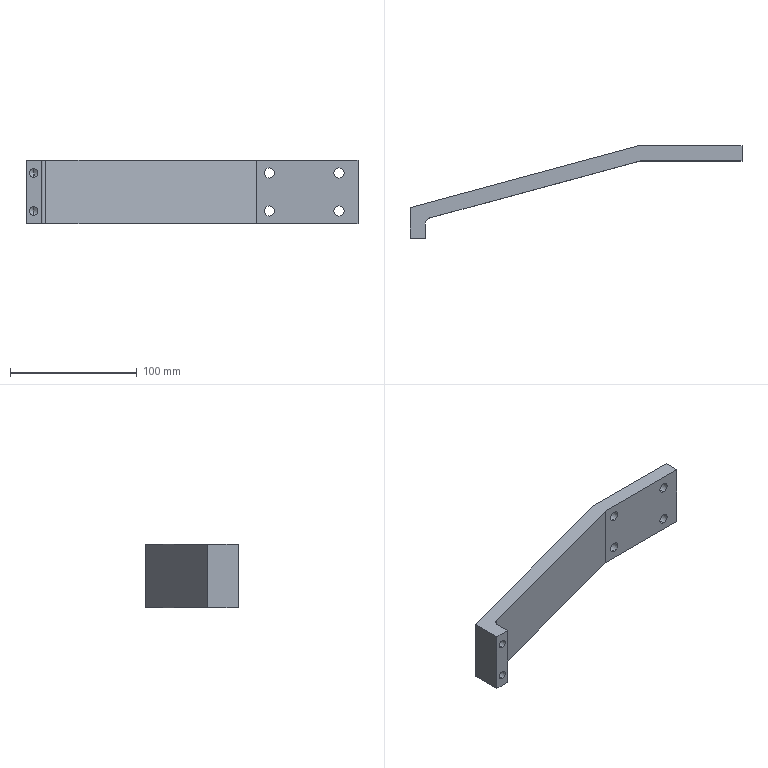Part | SolidWorks | features BaseBody 1 | 1 solid | 27 faces | box 262 x 73 x 50 mm | volume 165869 mm3 | cylinder 13 | plane 10 | cone 4 | commonest cylinder face diameters 8 x8 6.8 x4 10 x1
STEP:
#1=CARTESIAN_POINT('',(260.,-92.,221.121));
#2=VERTEX_POINT('',#1);
#3=CARTESIAN_POINT('',(260.,-92.,213.121));
#4=VERTEX_POINT('',#3);
#5=CARTESIAN_POINT('',(260.,-92.,217.121));
#6=DIRECTION('',(0.,-1.,0.));
#7=DIRECTION('',(0.,0.,1.));
#8=AXIS2_PLACEMENT_3D('',#5,#6,#7);
#9=CIRCLE('',#8,4.);
#10=EDGE_CURVE('',#2,#4,#9,.T.);
#11=ORIENTED_EDGE('',*,*,#10,.T.);
#12=CARTESIAN_POINT('',(260.,-80.,213.121));
#13=VERTEX_POINT('',#12);
#14=CARTESIAN_POINT('',(260.,-153.,213.121));
#15=DIRECTION('',(0.,1.,0.));
#16=VECTOR('',#15,1000.);
#17=LINE('',#14,#16);
#18=EDGE_CURVE('',#4,#13,#17,.T.);
#19=ORIENTED_EDGE('',*,*,#18,.T.);
#20=CARTESIAN_POINT('',(260.,-80.,221.121));
#21=VERTEX_POINT('',#20);
#22=CARTESIAN_POINT('',(260.,-80.,217.121));
#23=DIRECTION('',(0.,1.,0.));
#24=DIRECTION('',(0.,0.,1.));
#25=AXIS2_PLACEMENT_3D('',#22,#23,#24);
#26=CIRCLE('',#25,4.);
#27=EDGE_CURVE('',#13,#21,#26,.T.);
#28=ORIENTED_EDGE('',*,*,#27,.T.);
#29=CARTESIAN_POINT('',(260.,-153.,221.121));
#30=DIRECTION('',(0.,1.,0.));
#31=VECTOR('',#30,1000.);
#32=LINE('',#29,#31);
#33=EDGE_CURVE('',#2,#21,#32,.T.);
#34=ORIENTED_EDGE('',*,*,#33,.F.);
#35=EDGE_LOOP('',(#11,#19,#28,#34));
#36=FACE_OUTER_BOUND('',#35,.T.);
#37=CARTESIAN_POINT('',(260.,-153.,217.121));
#38=DIRECTION('',(0.,1.,0.));
#39=DIRECTION('',(0.,0.,1.));
#40=AXIS2_PLACEMENT_3D('',#37,#38,#39);
#41=CYLINDRICAL_SURFACE('',#40,4.);
#42=ADVANCED_FACE('',(#36),#41,.F.);
#43=CARTESIAN_POINT('',(260.,-92.,251.121));
#44=VERTEX_POINT('',#43);
#45=CARTESIAN_POINT('',(260.,-92.,243.121));
#46=VERTEX_POINT('',#45);
#47=CARTESIAN_POINT('',(260.,-92.,247.121));
#48=DIRECTION('',(0.,-1.,0.));
#49=DIRECTION('',(0.,0.,1.));
#50=AXIS2_PLACEMENT_3D('',#47,#48,#49);
#51=CIRCLE('',#50,4.);
#52=EDGE_CURVE('',#44,#46,#51,.T.);
#53=ORIENTED_EDGE('',*,*,#52,.T.);
#54=CARTESIAN_POINT('',(260.,-80.,243.121));
#55=VERTEX_POINT('',#54);
#56=CARTESIAN_POINT('',(260.,-153.,243.121));
#57=DIRECTION('',(0.,1.,0.));
#58=VECTOR('',#57,1000.);
#59=LINE('',#56,#58);
#60=EDGE_CURVE('',#46,#55,#59,.T.);
#61=ORIENTED_EDGE('',*,*,#60,.T.);
#62=CARTESIAN_POINT('',(260.,-80.,251.121));
#63=VERTEX_POINT('',#62);
#64=CARTESIAN_POINT('',(260.,-80.,247.121));
#65=DIRECTION('',(0.,1.,0.));
#66=DIRECTION('',(0.,0.,1.));
#67=AXIS2_PLACEMENT_3D('',#64,#65,#66);
#68=CIRCLE('',#67,4.);
#69=EDGE_CURVE('',#55,#63,#68,.T.);
#70=ORIENTED_EDGE('',*,*,#69,.T.);
#71=CARTESIAN_POINT('',(260.,-153.,251.121));
#72=DIRECTION('',(0.,1.,0.));
#73=VECTOR('',#72,1000.);
#74=LINE('',#71,#73);
#75=EDGE_CURVE('',#44,#63,#74,.T.);
#76=ORIENTED_EDGE('',*,*,#75,.F.);
#77=EDGE_LOOP('',(#53,#61,#70,#76));
#78=FACE_OUTER_BOUND('',#77,.T.);
#79=CARTESIAN_POINT('',(260.,-153.,247.121));
#80=DIRECTION('',(0.,1.,0.));
#81=DIRECTION('',(0.,0.,1.));
#82=AXIS2_PLACEMENT_3D('',#79,#80,#81);
#83=CYLINDRICAL_SURFACE('',#82,4.);
#84=ADVANCED_FACE('',(#78),#83,.F.);
#85=CARTESIAN_POINT('',(315.,-92.,251.121));
#86=VERTEX_POINT('',#85);
#87=CARTESIAN_POINT('',(315.,-92.,243.121));
#88=VERTEX_POINT('',#87);
#89=CARTESIAN_POINT('',(315.,-92.,247.121));
#90=DIRECTION('',(0.,-1.,0.));
#91=DIRECTION('',(0.,0.,1.));
#92=AXIS2_PLACEMENT_3D('',#89,#90,#91);
#93=CIRCLE('',#92,4.);
#94=EDGE_CURVE('',#86,#88,#93,.T.);
#95=ORIENTED_EDGE('',*,*,#94,.T.);
#96=CARTESIAN_POINT('',(315.,-80.,243.121));
#97=VERTEX_POINT('',#96);
#98=CARTESIAN_POINT('',(315.,-153.,243.121));
#99=DIRECTION('',(0.,1.,0.));
#100=VECTOR('',#99,1000.);
#101=LINE('',#98,#100);
#102=EDGE_CURVE('',#88,#97,#101,.T.);
#103=ORIENTED_EDGE('',*,*,#102,.T.);
#104=CARTESIAN_POINT('',(315.,-80.,251.121));
#105=VERTEX_POINT('',#104);
#106=CARTESIAN_POINT('',(315.,-80.,247.121));
#107=DIRECTION('',(0.,1.,0.));
#108=DIRECTION('',(0.,0.,1.));
#109=AXIS2_PLACEMENT_3D('',#106,#107,#108);
#110=CIRCLE('',#109,4.);
#111=EDGE_CURVE('',#97,#105,#110,.T.);
#112=ORIENTED_EDGE('',*,*,#111,.T.);
#113=CARTESIAN_POINT('',(315.,-153.,251.121));
#114=DIRECTION('',(0.,1.,0.));
#115=VECTOR('',#114,1000.);
#116=LINE('',#113,#115);
#117=EDGE_CURVE('',#86,#105,#116,.T.);
#118=ORIENTED_EDGE('',*,*,#117,.F.);
#119=EDGE_LOOP('',(#95,#103,#112,#118));
#120=FACE_OUTER_BOUND('',#119,.T.);
#121=CARTESIAN_POINT('',(315.,-153.,247.121));
#122=DIRECTION('',(0.,1.,0.));
#123=DIRECTION('',(0.,0.,1.));
#124=AXIS2_PLACEMENT_3D('',#121,#122,#123);
#125=CYLINDRICAL_SURFACE('',#124,4.);
#126=ADVANCED_FACE('',(#120),#125,.F.);
#127=CARTESIAN_POINT('',(315.,-92.,221.121));
#128=VERTEX_POINT('',#127);
#129=CARTESIAN_POINT('',(315.,-92.,213.121));
#130=VERTEX_POINT('',#129);
#131=CARTESIAN_POINT('',(315.,-92.,217.121));
#132=DIRECTION('',(0.,-1.,0.));
#133=DIRECTION('',(0.,0.,1.));
#134=AXIS2_PLACEMENT_3D('',#131,#132,#133);
#135=CIRCLE('',#134,4.);
#136=EDGE_CURVE('',#128,#130,#135,.T.);
#137=ORIENTED_EDGE('',*,*,#136,.T.);
#138=CARTESIAN_POINT('',(315.,-80.,213.121));
#139=VERTEX_POINT('',#138);
#140=CARTESIAN_POINT('',(315.,-153.,213.121));
#141=DIRECTION('',(0.,1.,0.));
#142=VECTOR('',#141,1000.);
#143=LINE('',#140,#142);
#144=EDGE_CURVE('',#130,#139,#143,.T.);
#145=ORIENTED_EDGE('',*,*,#144,.T.);
#146=CARTESIAN_POINT('',(315.,-80.,221.121));
#147=VERTEX_POINT('',#146);
#148=CARTESIAN_POINT('',(315.,-80.,217.121));
#149=DIRECTION('',(0.,1.,0.));
#150=DIRECTION('',(0.,0.,1.));
#151=AXIS2_PLACEMENT_3D('',#148,#149,#150);
#152=CIRCLE('',#151,4.);
#153=EDGE_CURVE('',#139,#147,#152,.T.);
#154=ORIENTED_EDGE('',*,*,#153,.T.);
#155=CARTESIAN_POINT('',(315.,-153.,221.121));
#156=DIRECTION('',(0.,1.,0.));
#157=VECTOR('',#156,1000.);
#158=LINE('',#155,#157);
#159=EDGE_CURVE('',#128,#147,#158,.T.);
#160=ORIENTED_EDGE('',*,*,#159,.F.);
#161=EDGE_LOOP('',(#137,#145,#154,#160));
#162=FACE_OUTER_BOUND('',#161,.T.);
#163=CARTESIAN_POINT('',(315.,-153.,217.121));
#164=DIRECTION('',(0.,1.,0.));
#165=DIRECTION('',(0.,0.,1.));
#166=AXIS2_PLACEMENT_3D('',#163,#164,#165);
#167=CYLINDRICAL_SURFACE('',#166,4.);
#168=ADVANCED_FACE('',(#162),#167,.F.);
#169=CARTESIAN_POINT('',(74.,-140.,250.521));
#170=VERTEX_POINT('',#169);
#171=CARTESIAN_POINT('',(74.,-140.,243.721));
#172=VERTEX_POINT('',#171);
#173=CARTESIAN_POINT('',(74.,-140.,247.121));
#174=DIRECTION('',(0.,-1.,0.));
#175=DIRECTION('',(0.,0.,-1.));
#176=AXIS2_PLACEMENT_3D('',#173,#174,#175);
#177=CIRCLE('',#176,3.4);
#178=EDGE_CURVE('',#170,#172,#177,.T.);
#179=ORIENTED_EDGE('',*,*,#178,.F.);
#180=CARTESIAN_POINT('',(74.,-153.,250.521));
#181=VERTEX_POINT('',#180);
#182=CARTESIAN_POINT('',(74.,-153.,250.521));
#183=DIRECTION('',(0.,-1.,0.));
#184=VECTOR('',#183,1000.);
#185=LINE('',#182,#184);
#186=EDGE_CURVE('',#170,#181,#185,.T.);
#187=ORIENTED_EDGE('',*,*,#186,.T.);
#188=CARTESIAN_POINT('',(74.,-153.,243.721));
#189=VERTEX_POINT('',#188);
#190=CARTESIAN_POINT('',(74.,-153.,247.121));
#191=DIRECTION('',(0.,-1.,0.));
#192=DIRECTION('',(0.,0.,-1.));
#193=AXIS2_PLACEMENT_3D('',#190,#191,#192);
#194=CIRCLE('',#193,3.4);
#195=EDGE_CURVE('',#181,#189,#194,.T.);
#196=ORIENTED_EDGE('',*,*,#195,.T.);
#197=CARTESIAN_POINT('',(74.,-153.,243.721));
#198=DIRECTION('',(0.,-1.,0.));
#199=VECTOR('',#198,1000.);
#200=LINE('',#197,#199);
#201=EDGE_CURVE('',#172,#189,#200,.T.);
#202=ORIENTED_EDGE('',*,*,#201,.F.);
#203=EDGE_LOOP('',(#179,#187,#196,#202));
#204=FACE_OUTER_BOUND('',#203,.T.);
#205=CARTESIAN_POINT('',(74.,-153.,247.121));
#206=DIRECTION('',(0.,-1.,0.));
#207=DIRECTION('',(0.,0.,-1.));
#208=AXIS2_PLACEMENT_3D('',#205,#206,#207);
#209=CYLINDRICAL_SURFACE('',#208,3.4);
#210=ADVANCED_FACE('',(#204),#209,.F.);
#211=CARTESIAN_POINT('',(74.,-140.,220.521));
#212=VERTEX_POINT('',#211);
#213=CARTESIAN_POINT('',(74.,-140.,213.721));
#214=VERTEX_POINT('',#213);
#215=CARTESIAN_POINT('',(74.,-140.,217.121));
#216=DIRECTION('',(0.,-1.,0.));
#217=DIRECTION('',(0.,0.,-1.));
#218=AXIS2_PLACEMENT_3D('',#215,#216,#217);
#219=CIRCLE('',#218,3.4);
#220=EDGE_CURVE('',#212,#214,#219,.T.);
#221=ORIENTED_EDGE('',*,*,#220,.F.);
#222=CARTESIAN_POINT('',(74.,-153.,220.521));
#223=VERTEX_POINT('',#222);
#224=CARTESIAN_POINT('',(74.,-153.,220.521));
#225=DIRECTION('',(0.,-1.,0.));
#226=VECTOR('',#225,1000.);
#227=LINE('',#224,#226);
#228=EDGE_CURVE('',#212,#223,#227,.T.);
#229=ORIENTED_EDGE('',*,*,#228,.T.);
#230=CARTESIAN_POINT('',(74.,-153.,213.721));
#231=VERTEX_POINT('',#230);
#232=CARTESIAN_POINT('',(74.,-153.,217.121));
#233=DIRECTION('',(0.,-1.,0.));
#234=DIRECTION('',(0.,0.,-1.));
#235=AXIS2_PLACEMENT_3D('',#232,#233,#234);
#236=CIRCLE('',#235,3.4);
#237=EDGE_CURVE('',#223,#231,#236,.T.);
#238=ORIENTED_EDGE('',*,*,#237,.T.);
#239=CARTESIAN_POINT('',(74.,-153.,213.721));
#240=DIRECTION('',(0.,-1.,0.));
#241=VECTOR('',#240,1000.);
#242=LINE('',#239,#241);
#243=EDGE_CURVE('',#214,#231,#242,.T.);
#244=ORIENTED_EDGE('',*,*,#243,.F.);
#245=EDGE_LOOP('',(#221,#229,#238,#244));
#246=FACE_OUTER_BOUND('',#245,.T.);
#247=CARTESIAN_POINT('',(74.,-153.,217.121));
#248=DIRECTION('',(0.,-1.,0.));
#249=DIRECTION('',(0.,0.,-1.));
#250=AXIS2_PLACEMENT_3D('',#247,#248,#249);
#251=CYLINDRICAL_SURFACE('',#250,3.4);
#252=ADVANCED_FACE('',(#246),#251,.F.);
#253=CARTESIAN_POINT('',(74.,-137.957,247.121));
#254=VERTEX_POINT('',#253);
#255=CARTESIAN_POINT('',(74.,-140.,243.721));
#256=DIRECTION('',(0.,-0.515,-0.8572));
#257=VECTOR('',#256,1000.);
#258=LINE('',#255,#257);
#259=EDGE_CURVE('',#254,#172,#258,.T.);
#260=ORIENTED_EDGE('',*,*,#259,.F.);
#261=CARTESIAN_POINT('',(74.,-140.,250.521));
#262=DIRECTION('',(0.,-0.515,0.8572));
#263=VECTOR('',#262,1000.);
#264=LINE('',#261,#263);
#265=EDGE_CURVE('',#254,#170,#264,.T.);
#266=ORIENTED_EDGE('',*,*,#265,.T.);
#267=ORIENTED_EDGE('',*,*,#178,.T.);
#268=EDGE_LOOP('',(#260,#266,#267));
#269=FACE_OUTER_BOUND('',#268,.T.);
#270=CARTESIAN_POINT('',(74.,-140.,247.121));
#271=DIRECTION('',(0.,-1.,0.));
#272=DIRECTION('',(0.,0.,-1.));
#273=AXIS2_PLACEMENT_3D('',#270,#271,#272);
#274=CONICAL_SURFACE('',#273,3.4,1.03);
#275=ADVANCED_FACE('',(#269),#274,.F.);
#276=CARTESIAN_POINT('',(74.,-137.957,217.121));
#277=VERTEX_POINT('',#276);
#278=CARTESIAN_POINT('',(74.,-140.,213.721));
#279=DIRECTION('',(0.,-0.515,-0.8572));
#280=VECTOR('',#279,1000.);
#281=LINE('',#278,#280);
#282=EDGE_CURVE('',#277,#214,#281,.T.);
#283=ORIENTED_EDGE('',*,*,#282,.F.);
#284=CARTESIAN_POINT('',(74.,-140.,220.521));
#285=DIRECTION('',(0.,-0.515,0.8572));
#286=VECTOR('',#285,1000.);
#287=LINE('',#284,#286);
#288=EDGE_CURVE('',#277,#212,#287,.T.);
#289=ORIENTED_EDGE('',*,*,#288,.T.);
#290=ORIENTED_EDGE('',*,*,#220,.T.);
#291=EDGE_LOOP('',(#283,#289,#290));
#292=FACE_OUTER_BOUND('',#291,.T.);
#293=CARTESIAN_POINT('',(74.,-140.,217.121));
#294=DIRECTION('',(0.,-1.,0.));
#295=DIRECTION('',(0.,0.,-1.));
#296=AXIS2_PLACEMENT_3D('',#293,#294,#295);
#297=CONICAL_SURFACE('',#296,3.4,1.03);
#298=ADVANCED_FACE('',(#292),#297,.F.);
#299=CARTESIAN_POINT('',(248.405,-80.,207.121));
#300=VERTEX_POINT('',#299);
#301=CARTESIAN_POINT('',(248.405,-80.,257.121));
#302=VERTEX_POINT('',#301);
#303=CARTESIAN_POINT('',(248.405,-80.,207.121));
#304=DIRECTION('',(0.,0.,1.));
#305=VECTOR('',#304,1000.);
#306=LINE('',#303,#305);
#307=EDGE_CURVE('',#300,#302,#306,.T.);
#308=ORIENTED_EDGE('',*,*,#307,.F.);
#309=CARTESIAN_POINT('',(68.,-128.816,207.121));
#310=VERTEX_POINT('',#309);
#311=CARTESIAN_POINT('',(68.,-128.816,207.121));
#312=DIRECTION('',(0.9653,0.2612,0.));
#313=VECTOR('',#312,1000.);
#314=LINE('',#311,#313);
#315=EDGE_CURVE('',#310,#300,#314,.T.);
#316=ORIENTED_EDGE('',*,*,#315,.F.);
#317=CARTESIAN_POINT('',(68.,-128.816,257.121));
#318=VERTEX_POINT('',#317);
#319=CARTESIAN_POINT('',(68.,-128.816,207.121));
#320=DIRECTION('',(0.,0.,-1.));
#321=VECTOR('',#320,1000.);
#322=LINE('',#319,#321);
#323=EDGE_CURVE('',#318,#310,#322,.T.);
#324=ORIENTED_EDGE('',*,*,#323,.F.);
#325=CARTESIAN_POINT('',(68.,-128.816,257.121));
#326=DIRECTION('',(-0.9653,-0.2612,0.));
#327=VECTOR('',#326,1000.);
#328=LINE('',#325,#327);
#329=EDGE_CURVE('',#302,#318,#328,.T.);
#330=ORIENTED_EDGE('',*,*,#329,.F.);
#331=EDGE_LOOP('',(#308,#316,#324,#330));
#332=FACE_OUTER_BOUND('',#331,.T.);
#333=CARTESIAN_POINT('',(68.,-128.816,207.121));
#334=DIRECTION('',(0.2612,-0.9653,0.));
#335=DIRECTION('',(0.9653,0.2612,0.));
#336=AXIS2_PLACEMENT_3D('',#333,#334,#335);
#337=PLANE('',#336);
#338=ADVANCED_FACE('',(#332),#337,.F.);
#339=CARTESIAN_POINT('',(80.,-141.827,257.121));
#340=VERTEX_POINT('',#339);
#341=CARTESIAN_POINT('',(80.,-153.,257.121));
#342=VERTEX_POINT('',#341);
#343=CARTESIAN_POINT('',(80.,-108.6,257.121));
#344=DIRECTION('',(0.,-1.,0.));
#345=VECTOR('',#344,1000.);
#346=LINE('',#343,#345);
#347=EDGE_CURVE('',#340,#342,#346,.T.);
#348=ORIENTED_EDGE('',*,*,#347,.F.);
#349=CARTESIAN_POINT('',(83.694,-137.,257.121));
#350=VERTEX_POINT('',#349);
#351=CARTESIAN_POINT('',(85.,-141.827,257.121));
#352=DIRECTION('',(0.,0.,1.));
#353=DIRECTION('',(-1.,0.,0.));
#354=AXIS2_PLACEMENT_3D('',#351,#352,#353);
#355=CIRCLE('',#354,5.);
#356=EDGE_CURVE('',#350,#340,#355,.T.);
#357=ORIENTED_EDGE('',*,*,#356,.F.);
#358=CARTESIAN_POINT('',(250.,-92.,257.121));
#359=VERTEX_POINT('',#358);
#360=CARTESIAN_POINT('',(250.,-92.,257.121));
#361=DIRECTION('',(-0.9653,-0.2612,0.));
#362=VECTOR('',#361,1000.);
#363=LINE('',#360,#362);
#364=EDGE_CURVE('',#359,#350,#363,.T.);
#365=ORIENTED_EDGE('',*,*,#364,.F.);
#366=CARTESIAN_POINT('',(330.,-92.,257.121));
#367=VERTEX_POINT('',#366);
#368=CARTESIAN_POINT('',(68.,-92.,257.121));
#369=DIRECTION('',(-1.,0.,0.));
#370=VECTOR('',#369,1000.);
#371=LINE('',#368,#370);
#372=EDGE_CURVE('',#367,#359,#371,.T.);
#373=ORIENTED_EDGE('',*,*,#372,.F.);
#374=CARTESIAN_POINT('',(330.,-80.,257.121));
#375=VERTEX_POINT('',#374);
#376=CARTESIAN_POINT('',(330.,-108.6,257.121));
#377=DIRECTION('',(0.,-1.,0.));
#378=VECTOR('',#377,1000.);
#379=LINE('',#376,#378);
#380=EDGE_CURVE('',#375,#367,#379,.T.);
#381=ORIENTED_EDGE('',*,*,#380,.F.);
#382=CARTESIAN_POINT('',(68.,-80.,257.121));
#383=DIRECTION('',(1.,0.,0.));
#384=VECTOR('',#383,1000.);
#385=LINE('',#382,#384);
#386=EDGE_CURVE('',#302,#375,#385,.T.);
#387=ORIENTED_EDGE('',*,*,#386,.F.);
#388=ORIENTED_EDGE('',*,*,#329,.T.);
#389=CARTESIAN_POINT('',(68.,-153.,257.121));
#390=VERTEX_POINT('',#389);
#391=CARTESIAN_POINT('',(68.,-108.6,257.121));
#392=DIRECTION('',(0.,1.,0.));
#393=VECTOR('',#392,1000.);
#394=LINE('',#391,#393);
#395=EDGE_CURVE('',#390,#318,#394,.T.);
#396=ORIENTED_EDGE('',*,*,#395,.F.);
#397=CARTESIAN_POINT('',(68.,-153.,257.121));
#398=DIRECTION('',(-1.,0.,0.));
#399=VECTOR('',#398,1000.);
#400=LINE('',#397,#399);
#401=EDGE_CURVE('',#342,#390,#400,.T.);
#402=ORIENTED_EDGE('',*,*,#401,.F.);
#403=EDGE_LOOP('',(#348,#357,#365,#373,#381,#387,#388,#396,#402));
#404=FACE_OUTER_BOUND('',#403,.T.);
#405=CARTESIAN_POINT('',(68.,-108.6,257.121));
#406=DIRECTION('',(0.,0.,-1.));
#407=DIRECTION('',(-1.,0.,0.));
#408=AXIS2_PLACEMENT_3D('',#405,#406,#407);
#409=PLANE('',#408);
#410=ADVANCED_FACE('',(#404),#409,.F.);
#411=CARTESIAN_POINT('',(330.,-80.,207.121));
#412=VERTEX_POINT('',#411);
#413=CARTESIAN_POINT('',(330.,-80.,207.121));
#414=DIRECTION('',(0.,0.,1.));
#415=VECTOR('',#414,1000.);
#416=LINE('',#413,#415);
#417=EDGE_CURVE('',#412,#375,#416,.T.);
#418=ORIENTED_EDGE('',*,*,#417,.F.);
#419=CARTESIAN_POINT('',(248.405,-80.,207.121));
#420=DIRECTION('',(1.,0.,0.));
#421=VECTOR('',#420,1000.);
#422=LINE('',#419,#421);
#423=EDGE_CURVE('',#300,#412,#422,.T.);
#424=ORIENTED_EDGE('',*,*,#423,.F.);
#425=ORIENTED_EDGE('',*,*,#307,.T.);
#426=ORIENTED_EDGE('',*,*,#386,.T.);
#427=EDGE_LOOP('',(#418,#424,#425,#426));
#428=FACE_OUTER_BOUND('',#427,.T.);
#429=CARTESIAN_POINT('',(260.,-80.,217.121));
#430=DIRECTION('',(0.,1.,0.));
#431=DIRECTION('',(0.,0.,1.));
#432=AXIS2_PLACEMENT_3D('',#429,#430,#431);
#433=CIRCLE('',#432,4.);
#434=EDGE_CURVE('',#21,#13,#433,.T.);
#435=ORIENTED_EDGE('',*,*,#434,.F.);
#436=ORIENTED_EDGE('',*,*,#27,.F.);
#437=EDGE_LOOP('',(#435,#436));
#438=FACE_BOUND('',#437,.T.);
#439=CARTESIAN_POINT('',(260.,-80.,247.121));
#440=DIRECTION('',(0.,1.,0.));
#441=DIRECTION('',(0.,0.,1.));
#442=AXIS2_PLACEMENT_3D('',#439,#440,#441);
#443=CIRCLE('',#442,4.);
#444=EDGE_CURVE('',#63,#55,#443,.T.);
#445=ORIENTED_EDGE('',*,*,#444,.F.);
#446=ORIENTED_EDGE('',*,*,#69,.F.);
#447=EDGE_LOOP('',(#445,#446));
#448=FACE_BOUND('',#447,.T.);
#449=CARTESIAN_POINT('',(315.,-80.,247.121));
#450=DIRECTION('',(0.,1.,0.));
#451=DIRECTION('',(0.,0.,1.));
#452=AXIS2_PLACEMENT_3D('',#449,#450,#451);
#453=CIRCLE('',#452,4.);
#454=EDGE_CURVE('',#105,#97,#453,.T.);
#455=ORIENTED_EDGE('',*,*,#454,.F.);
#456=ORIENTED_EDGE('',*,*,#111,.F.);
#457=EDGE_LOOP('',(#455,#456));
#458=FACE_BOUND('',#457,.T.);
#459=CARTESIAN_POINT('',(315.,-80.,217.121));
#460=DIRECTION('',(0.,1.,0.));
#461=DIRECTION('',(0.,0.,1.));
#462=AXIS2_PLACEMENT_3D('',#459,#460,#461);
#463=CIRCLE('',#462,4.);
#464=EDGE_CURVE('',#147,#139,#463,.T.);
#465=ORIENTED_EDGE('',*,*,#464,.F.);
#466=ORIENTED_EDGE('',*,*,#153,.F.);
#467=EDGE_LOOP('',(#465,#466));
#468=FACE_BOUND('',#467,.T.);
#469=CARTESIAN_POINT('',(248.405,-80.,207.121));
#470=DIRECTION('',(0.,-1.,0.));
#471=DIRECTION('',(0.,0.,-1.));
#472=AXIS2_PLACEMENT_3D('',#469,#470,#471);
#473=PLANE('',#472);
#474=ADVANCED_FACE('',(#428,#438,#448,#458,#468),#473,.F.);
#475=CARTESIAN_POINT('',(83.694,-137.,207.121));
#476=VERTEX_POINT('',#475);
#477=CARTESIAN_POINT('',(80.,-141.827,207.121));
#478=VERTEX_POINT('',#477);
#479=CARTESIAN_POINT('',(85.,-141.827,207.121));
#480=DIRECTION('',(0.,0.,1.));
#481=DIRECTION('',(-1.,0.,0.));
#482=AXIS2_PLACEMENT_3D('',#479,#480,#481);
#483=CIRCLE('',#482,5.);
#484=EDGE_CURVE('',#476,#478,#483,.T.);
#485=ORIENTED_EDGE('',*,*,#484,.T.);
#486=CARTESIAN_POINT('',(80.,-153.,207.121));
#487=VERTEX_POINT('',#486);
#488=CARTESIAN_POINT('',(80.,-108.6,207.121));
#489=DIRECTION('',(0.,-1.,0.));
#490=VECTOR('',#489,1000.);
#491=LINE('',#488,#490);
#492=EDGE_CURVE('',#478,#487,#491,.T.);
#493=ORIENTED_EDGE('',*,*,#492,.T.);
#494=CARTESIAN_POINT('',(68.,-153.,207.121));
#495=VERTEX_POINT('',#494);
#496=CARTESIAN_POINT('',(68.,-153.,207.121));
#497=DIRECTION('',(-1.,0.,0.));
#498=VECTOR('',#497,1000.);
#499=LINE('',#496,#498);
#500=EDGE_CURVE('',#487,#495,#499,.T.);
#501=ORIENTED_EDGE('',*,*,#500,.T.);
#502=CARTESIAN_POINT('',(68.,-108.6,207.121));
#503=DIRECTION('',(0.,1.,0.));
#504=VECTOR('',#503,1000.);
#505=LINE('',#502,#504);
#506=EDGE_CURVE('',#495,#310,#505,.T.);
#507=ORIENTED_EDGE('',*,*,#506,.T.);
#508=ORIENTED_EDGE('',*,*,#315,.T.);
#509=ORIENTED_EDGE('',*,*,#423,.T.);
#510=CARTESIAN_POINT('',(330.,-92.,207.121));
#511=VERTEX_POINT('',#510);
#512=CARTESIAN_POINT('',(330.,-108.6,207.121));
#513=DIRECTION('',(0.,-1.,0.));
#514=VECTOR('',#513,1000.);
#515=LINE('',#512,#514);
#516=EDGE_CURVE('',#412,#511,#515,.T.);
#517=ORIENTED_EDGE('',*,*,#516,.T.);
#518=CARTESIAN_POINT('',(250.,-92.,207.121));
#519=VERTEX_POINT('',#518);
#520=CARTESIAN_POINT('',(68.,-92.,207.121));
#521=DIRECTION('',(-1.,0.,0.));
#522=VECTOR('',#521,1000.);
#523=LINE('',#520,#522);
#524=EDGE_CURVE('',#511,#519,#523,.T.);
#525=ORIENTED_EDGE('',*,*,#524,.T.);
#526=CARTESIAN_POINT('',(250.,-92.,207.121));
#527=DIRECTION('',(-0.9653,-0.2612,0.));
#528=VECTOR('',#527,1000.);
#529=LINE('',#526,#528);
#530=EDGE_CURVE('',#519,#476,#529,.T.);
#531=ORIENTED_EDGE('',*,*,#530,.T.);
#532=EDGE_LOOP('',(#485,#493,#501,#507,#508,#509,#517,#525,#531));
#533=FACE_OUTER_BOUND('',#532,.T.);
#534=CARTESIAN_POINT('',(68.,-108.6,207.121));
#535=DIRECTION('',(0.,0.,-1.));
#536=DIRECTION('',(-1.,0.,0.));
#537=AXIS2_PLACEMENT_3D('',#534,#535,#536);
#538=PLANE('',#537);
#539=ADVANCED_FACE('',(#533),#538,.T.);
#540=ORIENTED_EDGE('',*,*,#323,.T.);
#541=ORIENTED_EDGE('',*,*,#506,.F.);
#542=CARTESIAN_POINT('',(68.,-153.,207.121));
#543=DIRECTION('',(0.,0.,-1.));
#544=VECTOR('',#543,1000.);
#545=LINE('',#542,#544);
#546=EDGE_CURVE('',#390,#495,#545,.T.);
#547=ORIENTED_EDGE('',*,*,#546,.F.);
#548=ORIENTED_EDGE('',*,*,#395,.T.);
#549=EDGE_LOOP('',(#540,#541,#547,#548));
#550=FACE_OUTER_BOUND('',#549,.T.);
#551=CARTESIAN_POINT('',(68.,-153.,207.121));
#552=DIRECTION('',(1.,0.,0.));
#553=DIRECTION('',(0.,0.,-1.));
#554=AXIS2_PLACEMENT_3D('',#551,#552,#553);
#555=PLANE('',#554);
#556=ADVANCED_FACE('',(#550),#555,.F.);
#557=ORIENTED_EDGE('',*,*,#546,.T.);
#558=ORIENTED_EDGE('',*,*,#500,.F.);
#559=CARTESIAN_POINT('',(80.,-153.,207.121));
#560=DIRECTION('',(0.,0.,-1.));
#561=VECTOR('',#560,1000.);
#562=LINE('',#559,#561);
#563=EDGE_CURVE('',#342,#487,#562,.T.);
#564=ORIENTED_EDGE('',*,*,#563,.F.);
#565=ORIENTED_EDGE('',*,*,#401,.T.);
#566=EDGE_LOOP('',(#557,#558,#564,#565));
#567=FACE_OUTER_BOUND('',#566,.T.);
#568=CARTESIAN_POINT('',(74.,-153.,247.121));
#569=DIRECTION('',(0.,-1.,0.));
#570=DIRECTION('',(0.,0.,-1.));
#571=AXIS2_PLACEMENT_3D('',#568,#569,#570);
#572=CIRCLE('',#571,3.4);
#573=EDGE_CURVE('',#189,#181,#572,.T.);
#574=ORIENTED_EDGE('',*,*,#573,.F.);
#575=ORIENTED_EDGE('',*,*,#195,.F.);
#576=EDGE_LOOP('',(#574,#575));
#577=FACE_BOUND('',#576,.T.);
#578=CARTESIAN_POINT('',(74.,-153.,217.121));
#579=DIRECTION('',(0.,-1.,0.));
#580=DIRECTION('',(0.,0.,-1.));
#581=AXIS2_PLACEMENT_3D('',#578,#579,#580);
#582=CIRCLE('',#581,3.4);
#583=EDGE_CURVE('',#231,#223,#582,.T.);
#584=ORIENTED_EDGE('',*,*,#583,.F.);
#585=ORIENTED_EDGE('',*,*,#237,.F.);
#586=EDGE_LOOP('',(#584,#585));
#587=FACE_BOUND('',#586,.T.);
#588=CARTESIAN_POINT('',(80.,-153.,207.121));
#589=DIRECTION('',(0.,1.,0.));
#590=DIRECTION('',(0.,0.,1.));
#591=AXIS2_PLACEMENT_3D('',#588,#589,#590);
#592=PLANE('',#591);
#593=ADVANCED_FACE('',(#567,#577,#587),#592,.F.);
#594=CARTESIAN_POINT('',(80.,-141.827,207.121));
#595=DIRECTION('',(0.,0.,-1.));
#596=VECTOR('',#595,1000.);
#597=LINE('',#594,#596);
#598=EDGE_CURVE('',#340,#478,#597,.T.);
#599=ORIENTED_EDGE('',*,*,#598,.F.);
#600=ORIENTED_EDGE('',*,*,#347,.T.);
#601=ORIENTED_EDGE('',*,*,#563,.T.);
#602=ORIENTED_EDGE('',*,*,#492,.F.);
#603=EDGE_LOOP('',(#599,#600,#601,#602));
#604=FACE_OUTER_BOUND('',#603,.T.);
#605=CARTESIAN_POINT('',(80.,-153.,207.121));
#606=DIRECTION('',(-1.,0.,0.));
#607=DIRECTION('',(0.,0.,1.));
#608=AXIS2_PLACEMENT_3D('',#605,#606,#607);
#609=PLANE('',#608);
#610=ADVANCED_FACE('',(#604),#609,.F.);
#611=CARTESIAN_POINT('',(83.694,-137.,207.121));
#612=DIRECTION('',(0.,0.,-1.));
#613=VECTOR('',#612,1000.);
#614=LINE('',#611,#613);
#615=EDGE_CURVE('',#350,#476,#614,.T.);
#616=ORIENTED_EDGE('',*,*,#615,.F.);
#617=ORIENTED_EDGE('',*,*,#356,.T.);
#618=ORIENTED_EDGE('',*,*,#598,.T.);
#619=ORIENTED_EDGE('',*,*,#484,.F.);
#620=EDGE_LOOP('',(#616,#617,#618,#619));
#621=FACE_OUTER_BOUND('',#620,.T.);
#622=CARTESIAN_POINT('',(85.,-141.827,207.121));
#623=DIRECTION('',(0.,0.,-1.));
#624=DIRECTION('',(-1.,0.,0.));
#625=AXIS2_PLACEMENT_3D('',#622,#623,#624);
#626=CYLINDRICAL_SURFACE('',#625,5.);
#627=ADVANCED_FACE('',(#621),#626,.F.);
#628=ORIENTED_EDGE('',*,*,#615,.T.);
#629=ORIENTED_EDGE('',*,*,#530,.F.);
#630=CARTESIAN_POINT('',(250.,-92.,207.121));
#631=DIRECTION('',(0.,0.,-1.));
#632=VECTOR('',#631,1000.);
#633=LINE('',#630,#632);
#634=EDGE_CURVE('',#359,#519,#633,.T.);
#635=ORIENTED_EDGE('',*,*,#634,.F.);
#636=ORIENTED_EDGE('',*,*,#364,.T.);
#637=EDGE_LOOP('',(#628,#629,#635,#636));
#638=FACE_OUTER_BOUND('',#637,.T.);
#639=CARTESIAN_POINT('',(80.,-138.,207.121));
#640=DIRECTION('',(-0.2612,0.9653,0.));
#641=DIRECTION('',(-0.9653,-0.2612,0.));
#642=AXIS2_PLACEMENT_3D('',#639,#640,#641);
#643=PLANE('',#642);
#644=ADVANCED_FACE('',(#638),#643,.F.);
#645=ORIENTED_EDGE('',*,*,#634,.T.);
#646=ORIENTED_EDGE('',*,*,#524,.F.);
#647=CARTESIAN_POINT('',(330.,-92.,207.121));
#648=DIRECTION('',(0.,0.,-1.));
#649=VECTOR('',#648,1000.);
#650=LINE('',#647,#649);
#651=EDGE_CURVE('',#367,#511,#650,.T.);
#652=ORIENTED_EDGE('',*,*,#651,.F.);
#653=ORIENTED_EDGE('',*,*,#372,.T.);
#654=EDGE_LOOP('',(#645,#646,#652,#653));
#655=FACE_OUTER_BOUND('',#654,.T.);
#656=ORIENTED_EDGE('',*,*,#10,.F.);
#657=CARTESIAN_POINT('',(260.,-92.,217.121));
#658=DIRECTION('',(0.,-1.,0.));
#659=DIRECTION('',(0.,0.,1.));
#660=AXIS2_PLACEMENT_3D('',#657,#658,#659);
#661=CIRCLE('',#660,4.);
#662=EDGE_CURVE('',#4,#2,#661,.T.);
#663=ORIENTED_EDGE('',*,*,#662,.F.);
#664=EDGE_LOOP('',(#656,#663));
#665=FACE_BOUND('',#664,.T.);
#666=ORIENTED_EDGE('',*,*,#52,.F.);
#667=CARTESIAN_POINT('',(260.,-92.,247.121));
#668=DIRECTION('',(0.,-1.,0.));
#669=DIRECTION('',(0.,0.,1.));
#670=AXIS2_PLACEMENT_3D('',#667,#668,#669);
#671=CIRCLE('',#670,4.);
#672=EDGE_CURVE('',#46,#44,#671,.T.);
#673=ORIENTED_EDGE('',*,*,#672,.F.);
#674=EDGE_LOOP('',(#666,#673));
#675=FACE_BOUND('',#674,.T.);
#676=ORIENTED_EDGE('',*,*,#94,.F.);
#677=CARTESIAN_POINT('',(315.,-92.,247.121));
#678=DIRECTION('',(0.,-1.,0.));
#679=DIRECTION('',(0.,0.,1.));
#680=AXIS2_PLACEMENT_3D('',#677,#678,#679);
#681=CIRCLE('',#680,4.);
#682=EDGE_CURVE('',#88,#86,#681,.T.);
#683=ORIENTED_EDGE('',*,*,#682,.F.);
#684=EDGE_LOOP('',(#676,#683));
#685=FACE_BOUND('',#684,.T.);
#686=ORIENTED_EDGE('',*,*,#136,.F.);
#687=CARTESIAN_POINT('',(315.,-92.,217.121));
#688=DIRECTION('',(0.,-1.,0.));
#689=DIRECTION('',(0.,0.,1.));
#690=AXIS2_PLACEMENT_3D('',#687,#688,#689);
#691=CIRCLE('',#690,4.);
#692=EDGE_CURVE('',#130,#128,#691,.T.);
#693=ORIENTED_EDGE('',*,*,#692,.F.);
#694=EDGE_LOOP('',(#686,#693));
#695=FACE_BOUND('',#694,.T.);
#696=CARTESIAN_POINT('',(250.,-92.,207.121));
#697=DIRECTION('',(0.,1.,0.));
#698=DIRECTION('',(0.,0.,1.));
#699=AXIS2_PLACEMENT_3D('',#696,#697,#698);
#700=PLANE('',#699);
#701=ADVANCED_FACE('',(#655,#665,#675,#685,#695),#700,.F.);
#702=ORIENTED_EDGE('',*,*,#651,.T.);
#703=ORIENTED_EDGE('',*,*,#516,.F.);
#704=ORIENTED_EDGE('',*,*,#417,.T.);
#705=ORIENTED_EDGE('',*,*,#380,.T.);
#706=EDGE_LOOP('',(#702,#703,#704,#705));
#707=FACE_OUTER_BOUND('',#706,.T.);
#708=CARTESIAN_POINT('',(330.,-80.,207.121));
#709=DIRECTION('',(-1.,0.,0.));
#710=DIRECTION('',(0.,0.,1.));
#711=AXIS2_PLACEMENT_3D('',#708,#709,#710);
#712=PLANE('',#711);
#713=ADVANCED_FACE('',(#707),#712,.F.);
#714=ORIENTED_EDGE('',*,*,#18,.F.);
#715=ORIENTED_EDGE('',*,*,#662,.T.);
#716=ORIENTED_EDGE('',*,*,#33,.T.);
#717=ORIENTED_EDGE('',*,*,#434,.T.);
#718=EDGE_LOOP('',(#714,#715,#716,#717));
#719=FACE_OUTER_BOUND('',#718,.T.);
#720=CARTESIAN_POINT('',(260.,-153.,217.121));
#721=DIRECTION('',(0.,1.,0.));
#722=DIRECTION('',(0.,0.,1.));
#723=AXIS2_PLACEMENT_3D('',#720,#721,#722);
#724=CYLINDRICAL_SURFACE('',#723,4.);
#725=ADVANCED_FACE('',(#719),#724,.F.);
#726=ORIENTED_EDGE('',*,*,#60,.F.);
#727=ORIENTED_EDGE('',*,*,#672,.T.);
#728=ORIENTED_EDGE('',*,*,#75,.T.);
#729=ORIENTED_EDGE('',*,*,#444,.T.);
#730=EDGE_LOOP('',(#726,#727,#728,#729));
#731=FACE_OUTER_BOUND('',#730,.T.);
#732=CARTESIAN_POINT('',(260.,-153.,247.121));
#733=DIRECTION('',(0.,1.,0.));
#734=DIRECTION('',(0.,0.,1.));
#735=AXIS2_PLACEMENT_3D('',#732,#733,#734);
#736=CYLINDRICAL_SURFACE('',#735,4.);
#737=ADVANCED_FACE('',(#731),#736,.F.);
#738=ORIENTED_EDGE('',*,*,#102,.F.);
#739=ORIENTED_EDGE('',*,*,#682,.T.);
#740=ORIENTED_EDGE('',*,*,#117,.T.);
#741=ORIENTED_EDGE('',*,*,#454,.T.);
#742=EDGE_LOOP('',(#738,#739,#740,#741));
#743=FACE_OUTER_BOUND('',#742,.T.);
#744=CARTESIAN_POINT('',(315.,-153.,247.121));
#745=DIRECTION('',(0.,1.,0.));
#746=DIRECTION('',(0.,0.,1.));
#747=AXIS2_PLACEMENT_3D('',#744,#745,#746);
#748=CYLINDRICAL_SURFACE('',#747,4.);
#749=ADVANCED_FACE('',(#743),#748,.F.);
#750=ORIENTED_EDGE('',*,*,#144,.F.);
#751=ORIENTED_EDGE('',*,*,#692,.T.);
#752=ORIENTED_EDGE('',*,*,#159,.T.);
#753=ORIENTED_EDGE('',*,*,#464,.T.);
#754=EDGE_LOOP('',(#750,#751,#752,#753));
#755=FACE_OUTER_BOUND('',#754,.T.);
#756=CARTESIAN_POINT('',(315.,-153.,217.121));
#757=DIRECTION('',(0.,1.,0.));
#758=DIRECTION('',(0.,0.,1.));
#759=AXIS2_PLACEMENT_3D('',#756,#757,#758);
#760=CYLINDRICAL_SURFACE('',#759,4.);
#761=ADVANCED_FACE('',(#755),#760,.F.);
#762=ORIENTED_EDGE('',*,*,#186,.F.);
#763=CARTESIAN_POINT('',(74.,-140.,247.121));
#764=DIRECTION('',(0.,-1.,0.));
#765=DIRECTION('',(0.,0.,-1.));
#766=AXIS2_PLACEMENT_3D('',#763,#764,#765);
#767=CIRCLE('',#766,3.4);
#768=EDGE_CURVE('',#172,#170,#767,.T.);
#769=ORIENTED_EDGE('',*,*,#768,.F.);
#770=ORIENTED_EDGE('',*,*,#201,.T.);
#771=ORIENTED_EDGE('',*,*,#573,.T.);
#772=EDGE_LOOP('',(#762,#769,#770,#771));
#773=FACE_OUTER_BOUND('',#772,.T.);
#774=CARTESIAN_POINT('',(74.,-153.,247.121));
#775=DIRECTION('',(0.,-1.,0.));
#776=DIRECTION('',(0.,0.,-1.));
#777=AXIS2_PLACEMENT_3D('',#774,#775,#776);
#778=CYLINDRICAL_SURFACE('',#777,3.4);
#779=ADVANCED_FACE('',(#773),#778,.F.);
#780=ORIENTED_EDGE('',*,*,#228,.F.);
#781=CARTESIAN_POINT('',(74.,-140.,217.121));
#782=DIRECTION('',(0.,-1.,0.));
#783=DIRECTION('',(0.,0.,-1.));
#784=AXIS2_PLACEMENT_3D('',#781,#782,#783);
#785=CIRCLE('',#784,3.4);
#786=EDGE_CURVE('',#214,#212,#785,.T.);
#787=ORIENTED_EDGE('',*,*,#786,.F.);
#788=ORIENTED_EDGE('',*,*,#243,.T.);
#789=ORIENTED_EDGE('',*,*,#583,.T.);
#790=EDGE_LOOP('',(#780,#787,#788,#789));
#791=FACE_OUTER_BOUND('',#790,.T.);
#792=CARTESIAN_POINT('',(74.,-153.,217.121));
#793=DIRECTION('',(0.,-1.,0.));
#794=DIRECTION('',(0.,0.,-1.));
#795=AXIS2_PLACEMENT_3D('',#792,#793,#794);
#796=CYLINDRICAL_SURFACE('',#795,3.4);
#797=ADVANCED_FACE('',(#791),#796,.F.);
#798=ORIENTED_EDGE('',*,*,#265,.F.);
#799=ORIENTED_EDGE('',*,*,#259,.T.);
#800=ORIENTED_EDGE('',*,*,#768,.T.);
#801=EDGE_LOOP('',(#798,#799,#800));
#802=FACE_OUTER_BOUND('',#801,.T.);
#803=CARTESIAN_POINT('',(74.,-140.,247.121));
#804=DIRECTION('',(0.,-1.,0.));
#805=DIRECTION('',(0.,0.,-1.));
#806=AXIS2_PLACEMENT_3D('',#803,#804,#805);
#807=CONICAL_SURFACE('',#806,3.4,1.03);
#808=ADVANCED_FACE('',(#802),#807,.F.);
#809=ORIENTED_EDGE('',*,*,#288,.F.);
#810=ORIENTED_EDGE('',*,*,#282,.T.);
#811=ORIENTED_EDGE('',*,*,#786,.T.);
#812=EDGE_LOOP('',(#809,#810,#811));
#813=FACE_OUTER_BOUND('',#812,.T.);
#814=CARTESIAN_POINT('',(74.,-140.,217.121));
#815=DIRECTION('',(0.,-1.,0.));
#816=DIRECTION('',(0.,0.,-1.));
#817=AXIS2_PLACEMENT_3D('',#814,#815,#816);
#818=CONICAL_SURFACE('',#817,3.4,1.03);
#819=ADVANCED_FACE('',(#813),#818,.F.);
#820=CLOSED_SHELL('',(#42,#84,#126,#168,#210,#252,#275,#298,#338,#410,#474,#539,#556,#593,#610,#627,#644,#701,#713,#725,#737,#749,#761,#779,#797,#808,#819));
#821=MANIFOLD_SOLID_BREP('',#820);
#822=CARTESIAN_POINT('',(0.,0.,0.));
#823=DIRECTION('',(0.,0.,1.));
#824=DIRECTION('',(1.,0.,0.));
#825=AXIS2_PLACEMENT_3D('',#822,#823,#824);
#826=(LENGTH_UNIT()NAMED_UNIT(*)SI_UNIT(.MILLI.,.METRE.));
#827=UNCERTAINTY_MEASURE_WITH_UNIT(LENGTH_MEASURE(0.00001),#826,'','');
#828=(NAMED_UNIT(*)PLANE_ANGLE_UNIT()SI_UNIT($,.RADIAN.));
#829=(NAMED_UNIT(*)SI_UNIT($,.STERADIAN.)SOLID_ANGLE_UNIT());
#830=(GEOMETRIC_REPRESENTATION_CONTEXT(3)GLOBAL_UNCERTAINTY_ASSIGNED_CONTEXT((#827))GLOBAL_UNIT_ASSIGNED_CONTEXT((#826,#828,#829))REPRESENTATION_CONTEXT('',''));
#831=ADVANCED_BREP_SHAPE_REPRESENTATION('',(#821,#825),#830);